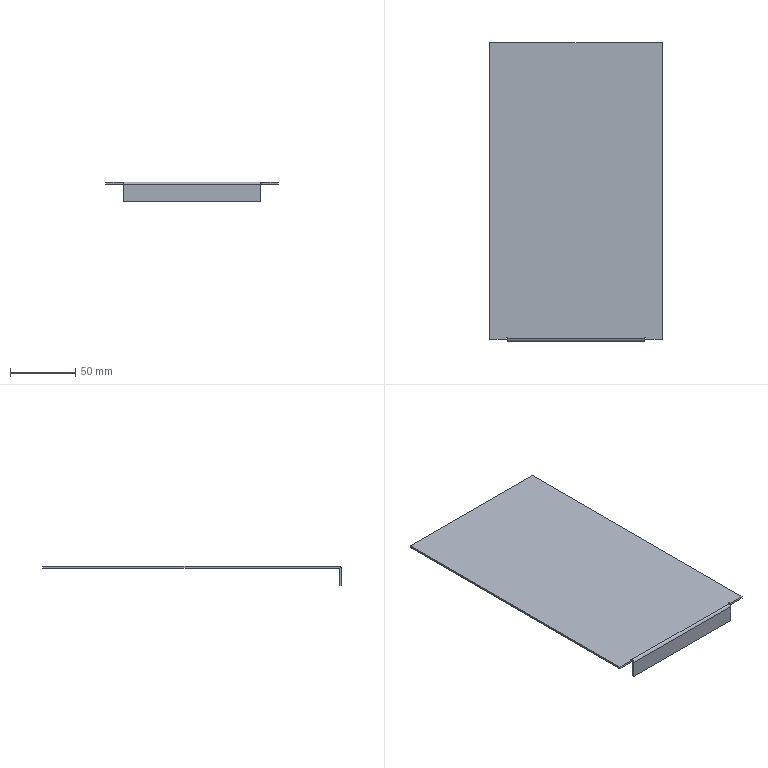Part | STEP file | X Motor Cover 1-1 | 1 solid | 18 faces | box 132 x 228.5 x 15 mm | volume 47221 mm3 | plane 14 | cylinder 4 | commonest cylinder face diameters 0.75 x2 1 x1 4 x1
STEP:
#1=CARTESIAN_POINT('',(-39.22,-140.718,-1.5));
#2=VERTEX_POINT('',#1);
#3=CARTESIAN_POINT('',(-26.47,-140.718,-1.5));
#4=VERTEX_POINT('',#3);
#5=CARTESIAN_POINT('',(0.,-140.718,-1.5));
#6=DIRECTION('',(1.,0.,0.));
#7=VECTOR('',#6,1000.);
#8=LINE('',#5,#7);
#9=EDGE_CURVE('',#2,#4,#8,.T.);
#10=ORIENTED_EDGE('',*,*,#9,.F.);
#11=CARTESIAN_POINT('',(-39.22,86.282,-1.5));
#12=VERTEX_POINT('',#11);
#13=CARTESIAN_POINT('',(-39.22,0.,-1.5));
#14=DIRECTION('',(0.,-1.,0.));
#15=VECTOR('',#14,1000.);
#16=LINE('',#13,#15);
#17=EDGE_CURVE('',#12,#2,#16,.T.);
#18=ORIENTED_EDGE('',*,*,#17,.F.);
#19=CARTESIAN_POINT('',(92.78,86.282,-1.5));
#20=VERTEX_POINT('',#19);
#21=CARTESIAN_POINT('',(0.,86.282,-1.5));
#22=DIRECTION('',(-1.,0.,0.));
#23=VECTOR('',#22,1000.);
#24=LINE('',#21,#23);
#25=EDGE_CURVE('',#20,#12,#24,.T.);
#26=ORIENTED_EDGE('',*,*,#25,.F.);
#27=CARTESIAN_POINT('',(92.78,-140.718,-1.5));
#28=VERTEX_POINT('',#27);
#29=CARTESIAN_POINT('',(92.78,0.,-1.5));
#30=DIRECTION('',(0.,1.,0.));
#31=VECTOR('',#30,1000.);
#32=LINE('',#29,#31);
#33=EDGE_CURVE('',#28,#20,#32,.T.);
#34=ORIENTED_EDGE('',*,*,#33,.F.);
#35=CARTESIAN_POINT('',(80.03,-140.718,-1.5));
#36=VERTEX_POINT('',#35);
#37=CARTESIAN_POINT('',(0.,-140.718,-1.5));
#38=DIRECTION('',(1.,0.,0.));
#39=VECTOR('',#38,1000.);
#40=LINE('',#37,#39);
#41=EDGE_CURVE('',#36,#28,#40,.T.);
#42=ORIENTED_EDGE('',*,*,#41,.F.);
#43=CARTESIAN_POINT('',(80.03,-139.468,-1.5));
#44=VERTEX_POINT('',#43);
#45=CARTESIAN_POINT('',(80.03,0.,-1.5));
#46=DIRECTION('',(0.,-1.,0.));
#47=VECTOR('',#46,1000.);
#48=LINE('',#45,#47);
#49=EDGE_CURVE('',#44,#36,#48,.T.);
#50=ORIENTED_EDGE('',*,*,#49,.F.);
#51=CARTESIAN_POINT('',(79.28,-139.468,-1.5));
#52=VERTEX_POINT('',#51);
#53=CARTESIAN_POINT('',(79.655,-139.468,-1.5));
#54=DIRECTION('',(0.,0.,-1.));
#55=DIRECTION('',(1.,0.,0.));
#56=AXIS2_PLACEMENT_3D('',#53,#54,#55);
#57=CIRCLE('',#56,0.375);
#58=EDGE_CURVE('',#52,#44,#57,.T.);
#59=ORIENTED_EDGE('',*,*,#58,.F.);
#60=CARTESIAN_POINT('',(79.28,-140.218,-1.5));
#61=VERTEX_POINT('',#60);
#62=CARTESIAN_POINT('',(79.28,-140.218,-1.5));
#63=DIRECTION('',(0.,1.,0.));
#64=VECTOR('',#63,1000.);
#65=LINE('',#62,#64);
#66=EDGE_CURVE('',#61,#52,#65,.T.);
#67=ORIENTED_EDGE('',*,*,#66,.F.);
#68=CARTESIAN_POINT('',(-25.72,-140.218,-1.5));
#69=VERTEX_POINT('',#68);
#70=CARTESIAN_POINT('',(0.,-140.218,-1.5));
#71=DIRECTION('',(1.,0.,0.));
#72=VECTOR('',#71,1000.);
#73=LINE('',#70,#72);
#74=EDGE_CURVE('',#69,#61,#73,.T.);
#75=ORIENTED_EDGE('',*,*,#74,.F.);
#76=CARTESIAN_POINT('',(-25.72,-139.468,-1.5));
#77=VERTEX_POINT('',#76);
#78=CARTESIAN_POINT('',(-25.72,0.,-1.5));
#79=DIRECTION('',(0.,-1.,0.));
#80=VECTOR('',#79,1000.);
#81=LINE('',#78,#80);
#82=EDGE_CURVE('',#77,#69,#81,.T.);
#83=ORIENTED_EDGE('',*,*,#82,.F.);
#84=CARTESIAN_POINT('',(-26.47,-139.468,-1.5));
#85=VERTEX_POINT('',#84);
#86=CARTESIAN_POINT('',(-26.095,-139.468,-1.5));
#87=DIRECTION('',(0.,0.,-1.));
#88=DIRECTION('',(1.,0.,0.));
#89=AXIS2_PLACEMENT_3D('',#86,#87,#88);
#90=CIRCLE('',#89,0.375);
#91=EDGE_CURVE('',#85,#77,#90,.T.);
#92=ORIENTED_EDGE('',*,*,#91,.F.);
#93=CARTESIAN_POINT('',(-26.47,0.,-1.5));
#94=DIRECTION('',(0.,1.,0.));
#95=VECTOR('',#94,1000.);
#96=LINE('',#93,#95);
#97=EDGE_CURVE('',#4,#85,#96,.T.);
#98=ORIENTED_EDGE('',*,*,#97,.F.);
#99=EDGE_LOOP('',(#10,#18,#26,#34,#42,#50,#59,#67,#75,#83,#92,#98));
#100=FACE_OUTER_BOUND('',#99,.T.);
#101=CARTESIAN_POINT('',(0.,0.,-1.5));
#102=DIRECTION('',(0.,0.,1.));
#103=DIRECTION('',(1.,0.,0.));
#104=AXIS2_PLACEMENT_3D('',#101,#102,#103);
#105=PLANE('',#104);
#106=ADVANCED_FACE('',(#100),#105,.F.);
#107=ORIENTED_EDGE('',*,*,#97,.T.);
#108=CARTESIAN_POINT('',(-26.47,-139.468,0.));
#109=VERTEX_POINT('',#108);
#110=CARTESIAN_POINT('',(-26.47,-139.468,-1.5));
#111=DIRECTION('',(0.,0.,1.));
#112=VECTOR('',#111,1000.);
#113=LINE('',#110,#112);
#114=EDGE_CURVE('',#85,#109,#113,.T.);
#115=ORIENTED_EDGE('',*,*,#114,.T.);
#116=CARTESIAN_POINT('',(-26.47,-140.718,0.));
#117=VERTEX_POINT('',#116);
#118=CARTESIAN_POINT('',(-26.47,0.,0.));
#119=DIRECTION('',(0.,1.,0.));
#120=VECTOR('',#119,1000.);
#121=LINE('',#118,#120);
#122=EDGE_CURVE('',#117,#109,#121,.T.);
#123=ORIENTED_EDGE('',*,*,#122,.F.);
#124=CARTESIAN_POINT('',(-26.47,-140.718,-1.5));
#125=DIRECTION('',(0.,0.,-1.));
#126=VECTOR('',#125,1000.);
#127=LINE('',#124,#126);
#128=EDGE_CURVE('',#117,#4,#127,.T.);
#129=ORIENTED_EDGE('',*,*,#128,.T.);
#130=EDGE_LOOP('',(#107,#115,#123,#129));
#131=FACE_OUTER_BOUND('',#130,.T.);
#132=CARTESIAN_POINT('',(-26.47,-140.718,-1.5));
#133=DIRECTION('',(1.,0.,0.));
#134=DIRECTION('',(0.,0.,-1.));
#135=AXIS2_PLACEMENT_3D('',#132,#133,#134);
#136=PLANE('',#135);
#137=ADVANCED_FACE('',(#131),#136,.T.);
#138=CARTESIAN_POINT('',(-39.22,-140.718,0.));
#139=VERTEX_POINT('',#138);
#140=CARTESIAN_POINT('',(-39.22,-140.718,0.));
#141=DIRECTION('',(-1.,0.,0.));
#142=VECTOR('',#141,1000.);
#143=LINE('',#140,#142);
#144=EDGE_CURVE('',#117,#139,#143,.T.);
#145=ORIENTED_EDGE('',*,*,#144,.T.);
#146=CARTESIAN_POINT('',(-39.22,-140.718,-1.5));
#147=DIRECTION('',(0.,0.,-1.));
#148=VECTOR('',#147,1000.);
#149=LINE('',#146,#148);
#150=EDGE_CURVE('',#139,#2,#149,.T.);
#151=ORIENTED_EDGE('',*,*,#150,.T.);
#152=ORIENTED_EDGE('',*,*,#9,.T.);
#153=ORIENTED_EDGE('',*,*,#128,.F.);
#154=EDGE_LOOP('',(#145,#151,#152,#153));
#155=FACE_OUTER_BOUND('',#154,.T.);
#156=CARTESIAN_POINT('',(-39.22,-140.718,-1.5));
#157=DIRECTION('',(0.,-1.,0.));
#158=DIRECTION('',(0.,0.,-1.));
#159=AXIS2_PLACEMENT_3D('',#156,#157,#158);
#160=PLANE('',#159);
#161=ADVANCED_FACE('',(#155),#160,.T.);
#162=ORIENTED_EDGE('',*,*,#17,.T.);
#163=ORIENTED_EDGE('',*,*,#150,.F.);
#164=CARTESIAN_POINT('',(-39.22,86.282,0.));
#165=VERTEX_POINT('',#164);
#166=CARTESIAN_POINT('',(-39.22,86.282,0.));
#167=DIRECTION('',(0.,1.,0.));
#168=VECTOR('',#167,1000.);
#169=LINE('',#166,#168);
#170=EDGE_CURVE('',#139,#165,#169,.T.);
#171=ORIENTED_EDGE('',*,*,#170,.T.);
#172=CARTESIAN_POINT('',(-39.22,86.282,-1.5));
#173=DIRECTION('',(0.,0.,-1.));
#174=VECTOR('',#173,1000.);
#175=LINE('',#172,#174);
#176=EDGE_CURVE('',#165,#12,#175,.T.);
#177=ORIENTED_EDGE('',*,*,#176,.T.);
#178=EDGE_LOOP('',(#162,#163,#171,#177));
#179=FACE_OUTER_BOUND('',#178,.T.);
#180=CARTESIAN_POINT('',(-39.22,86.282,-1.5));
#181=DIRECTION('',(-1.,0.,0.));
#182=DIRECTION('',(0.,-1.,0.));
#183=AXIS2_PLACEMENT_3D('',#180,#181,#182);
#184=PLANE('',#183);
#185=ADVANCED_FACE('',(#179),#184,.T.);
#186=ORIENTED_EDGE('',*,*,#25,.T.);
#187=ORIENTED_EDGE('',*,*,#176,.F.);
#188=CARTESIAN_POINT('',(92.78,86.282,0.));
#189=VERTEX_POINT('',#188);
#190=CARTESIAN_POINT('',(-39.22,86.282,0.));
#191=DIRECTION('',(1.,0.,0.));
#192=VECTOR('',#191,1000.);
#193=LINE('',#190,#192);
#194=EDGE_CURVE('',#165,#189,#193,.T.);
#195=ORIENTED_EDGE('',*,*,#194,.T.);
#196=CARTESIAN_POINT('',(92.78,86.282,-1.5));
#197=DIRECTION('',(0.,0.,-1.));
#198=VECTOR('',#197,1000.);
#199=LINE('',#196,#198);
#200=EDGE_CURVE('',#189,#20,#199,.T.);
#201=ORIENTED_EDGE('',*,*,#200,.T.);
#202=EDGE_LOOP('',(#186,#187,#195,#201));
#203=FACE_OUTER_BOUND('',#202,.T.);
#204=CARTESIAN_POINT('',(-39.22,86.282,-1.5));
#205=DIRECTION('',(0.,1.,0.));
#206=DIRECTION('',(0.,0.,1.));
#207=AXIS2_PLACEMENT_3D('',#204,#205,#206);
#208=PLANE('',#207);
#209=ADVANCED_FACE('',(#203),#208,.T.);
#210=ORIENTED_EDGE('',*,*,#33,.T.);
#211=ORIENTED_EDGE('',*,*,#200,.F.);
#212=CARTESIAN_POINT('',(92.78,-140.718,0.));
#213=VERTEX_POINT('',#212);
#214=CARTESIAN_POINT('',(92.78,86.282,0.));
#215=DIRECTION('',(0.,-1.,0.));
#216=VECTOR('',#215,1000.);
#217=LINE('',#214,#216);
#218=EDGE_CURVE('',#189,#213,#217,.T.);
#219=ORIENTED_EDGE('',*,*,#218,.T.);
#220=CARTESIAN_POINT('',(92.78,-140.718,-1.5));
#221=DIRECTION('',(0.,0.,-1.));
#222=VECTOR('',#221,1000.);
#223=LINE('',#220,#222);
#224=EDGE_CURVE('',#213,#28,#223,.T.);
#225=ORIENTED_EDGE('',*,*,#224,.T.);
#226=EDGE_LOOP('',(#210,#211,#219,#225));
#227=FACE_OUTER_BOUND('',#226,.T.);
#228=CARTESIAN_POINT('',(92.78,86.282,-1.5));
#229=DIRECTION('',(1.,0.,0.));
#230=DIRECTION('',(0.,1.,0.));
#231=AXIS2_PLACEMENT_3D('',#228,#229,#230);
#232=PLANE('',#231);
#233=ADVANCED_FACE('',(#227),#232,.T.);
#234=ORIENTED_EDGE('',*,*,#41,.T.);
#235=ORIENTED_EDGE('',*,*,#224,.F.);
#236=CARTESIAN_POINT('',(80.03,-140.718,0.));
#237=VERTEX_POINT('',#236);
#238=CARTESIAN_POINT('',(-39.22,-140.718,0.));
#239=DIRECTION('',(-1.,0.,0.));
#240=VECTOR('',#239,1000.);
#241=LINE('',#238,#240);
#242=EDGE_CURVE('',#213,#237,#241,.T.);
#243=ORIENTED_EDGE('',*,*,#242,.T.);
#244=CARTESIAN_POINT('',(80.03,-140.718,-1.5));
#245=DIRECTION('',(0.,0.,-1.));
#246=VECTOR('',#245,1000.);
#247=LINE('',#244,#246);
#248=EDGE_CURVE('',#237,#36,#247,.T.);
#249=ORIENTED_EDGE('',*,*,#248,.T.);
#250=EDGE_LOOP('',(#234,#235,#243,#249));
#251=FACE_OUTER_BOUND('',#250,.T.);
#252=CARTESIAN_POINT('',(-39.22,-140.718,-1.5));
#253=DIRECTION('',(0.,-1.,0.));
#254=DIRECTION('',(0.,0.,-1.));
#255=AXIS2_PLACEMENT_3D('',#252,#253,#254);
#256=PLANE('',#255);
#257=ADVANCED_FACE('',(#251),#256,.T.);
#258=ORIENTED_EDGE('',*,*,#49,.T.);
#259=ORIENTED_EDGE('',*,*,#248,.F.);
#260=CARTESIAN_POINT('',(80.03,-139.468,0.));
#261=VERTEX_POINT('',#260);
#262=CARTESIAN_POINT('',(80.03,-139.468,0.));
#263=DIRECTION('',(0.,1.,0.));
#264=VECTOR('',#263,1000.);
#265=LINE('',#262,#264);
#266=EDGE_CURVE('',#237,#261,#265,.T.);
#267=ORIENTED_EDGE('',*,*,#266,.T.);
#268=CARTESIAN_POINT('',(80.03,-139.468,-1.5));
#269=DIRECTION('',(0.,0.,-1.));
#270=VECTOR('',#269,1000.);
#271=LINE('',#268,#270);
#272=EDGE_CURVE('',#261,#44,#271,.T.);
#273=ORIENTED_EDGE('',*,*,#272,.T.);
#274=EDGE_LOOP('',(#258,#259,#267,#273));
#275=FACE_OUTER_BOUND('',#274,.T.);
#276=CARTESIAN_POINT('',(80.03,-139.468,-1.5));
#277=DIRECTION('',(-1.,0.,0.));
#278=DIRECTION('',(0.,0.,1.));
#279=AXIS2_PLACEMENT_3D('',#276,#277,#278);
#280=PLANE('',#279);
#281=ADVANCED_FACE('',(#275),#280,.T.);
#282=CARTESIAN_POINT('',(79.28,-139.468,0.));
#283=VERTEX_POINT('',#282);
#284=CARTESIAN_POINT('',(79.28,-139.468,-1.5));
#285=DIRECTION('',(0.,0.,1.));
#286=VECTOR('',#285,1000.);
#287=LINE('',#284,#286);
#288=EDGE_CURVE('',#52,#283,#287,.T.);
#289=ORIENTED_EDGE('',*,*,#288,.F.);
#290=ORIENTED_EDGE('',*,*,#58,.T.);
#291=ORIENTED_EDGE('',*,*,#272,.F.);
#292=CARTESIAN_POINT('',(79.655,-139.468,0.));
#293=DIRECTION('',(0.,0.,-1.));
#294=DIRECTION('',(1.,0.,0.));
#295=AXIS2_PLACEMENT_3D('',#292,#293,#294);
#296=CIRCLE('',#295,0.375);
#297=EDGE_CURVE('',#283,#261,#296,.T.);
#298=ORIENTED_EDGE('',*,*,#297,.F.);
#299=EDGE_LOOP('',(#289,#290,#291,#298));
#300=FACE_OUTER_BOUND('',#299,.T.);
#301=CARTESIAN_POINT('',(79.655,-139.468,-1.5));
#302=DIRECTION('',(0.,0.,1.));
#303=DIRECTION('',(1.,0.,0.));
#304=AXIS2_PLACEMENT_3D('',#301,#302,#303);
#305=CYLINDRICAL_SURFACE('',#304,0.375);
#306=ADVANCED_FACE('',(#300),#305,.F.);
#307=CARTESIAN_POINT('',(79.28,-140.718,-2.));
#308=VERTEX_POINT('',#307);
#309=CARTESIAN_POINT('',(79.28,-140.218,-2.));
#310=DIRECTION('',(-1.,0.,0.));
#311=DIRECTION('',(0.,0.,1.));
#312=AXIS2_PLACEMENT_3D('',#309,#310,#311);
#313=CIRCLE('',#312,0.5);
#314=EDGE_CURVE('',#308,#61,#313,.T.);
#315=ORIENTED_EDGE('',*,*,#314,.F.);
#316=CARTESIAN_POINT('',(-25.72,-140.718,-2.));
#317=VERTEX_POINT('',#316);
#318=CARTESIAN_POINT('',(-25.72,-140.718,-2.));
#319=DIRECTION('',(1.,0.,0.));
#320=VECTOR('',#319,1000.);
#321=LINE('',#318,#320);
#322=EDGE_CURVE('',#317,#308,#321,.T.);
#323=ORIENTED_EDGE('',*,*,#322,.F.);
#324=CARTESIAN_POINT('',(-25.72,-140.218,-2.));
#325=DIRECTION('',(-1.,0.,0.));
#326=DIRECTION('',(0.,0.,1.));
#327=AXIS2_PLACEMENT_3D('',#324,#325,#326);
#328=CIRCLE('',#327,0.5);
#329=EDGE_CURVE('',#317,#69,#328,.T.);
#330=ORIENTED_EDGE('',*,*,#329,.T.);
#331=ORIENTED_EDGE('',*,*,#74,.T.);
#332=EDGE_LOOP('',(#315,#323,#330,#331));
#333=FACE_OUTER_BOUND('',#332,.T.);
#334=CARTESIAN_POINT('',(-25.72,-140.218,-2.));
#335=DIRECTION('',(-1.,0.,0.));
#336=DIRECTION('',(0.,0.,1.));
#337=AXIS2_PLACEMENT_3D('',#334,#335,#336);
#338=CYLINDRICAL_SURFACE('',#337,0.5);
#339=ADVANCED_FACE('',(#333),#338,.F.);
#340=ORIENTED_EDGE('',*,*,#82,.T.);
#341=ORIENTED_EDGE('',*,*,#329,.F.);
#342=CARTESIAN_POINT('',(-25.72,-140.718,-15.));
#343=VERTEX_POINT('',#342);
#344=CARTESIAN_POINT('',(-25.72,-140.718,0.));
#345=DIRECTION('',(0.,0.,-1.));
#346=VECTOR('',#345,1000.);
#347=LINE('',#344,#346);
#348=EDGE_CURVE('',#317,#343,#347,.T.);
#349=ORIENTED_EDGE('',*,*,#348,.T.);
#350=CARTESIAN_POINT('',(-25.72,-142.218,-15.));
#351=VERTEX_POINT('',#350);
#352=CARTESIAN_POINT('',(-25.72,-142.218,-15.));
#353=DIRECTION('',(0.,1.,0.));
#354=VECTOR('',#353,1000.);
#355=LINE('',#352,#354);
#356=EDGE_CURVE('',#351,#343,#355,.T.);
#357=ORIENTED_EDGE('',*,*,#356,.F.);
#358=CARTESIAN_POINT('',(-25.72,-142.218,-2.));
#359=VERTEX_POINT('',#358);
#360=CARTESIAN_POINT('',(-25.72,-142.218,-1.5));
#361=DIRECTION('',(0.,0.,1.));
#362=VECTOR('',#361,1000.);
#363=LINE('',#360,#362);
#364=EDGE_CURVE('',#351,#359,#363,.T.);
#365=ORIENTED_EDGE('',*,*,#364,.T.);
#366=CARTESIAN_POINT('',(-25.72,-140.218,0.));
#367=VERTEX_POINT('',#366);
#368=CARTESIAN_POINT('',(-25.72,-140.218,-2.));
#369=DIRECTION('',(1.,0.,0.));
#370=DIRECTION('',(0.,0.,1.));
#371=AXIS2_PLACEMENT_3D('',#368,#369,#370);
#372=CIRCLE('',#371,2.);
#373=EDGE_CURVE('',#367,#359,#372,.T.);
#374=ORIENTED_EDGE('',*,*,#373,.F.);
#375=CARTESIAN_POINT('',(-25.72,-139.468,0.));
#376=VERTEX_POINT('',#375);
#377=CARTESIAN_POINT('',(-25.72,-139.468,0.));
#378=DIRECTION('',(0.,1.,0.));
#379=VECTOR('',#378,1000.);
#380=LINE('',#377,#379);
#381=EDGE_CURVE('',#367,#376,#380,.T.);
#382=ORIENTED_EDGE('',*,*,#381,.T.);
#383=CARTESIAN_POINT('',(-25.72,-139.468,-1.5));
#384=DIRECTION('',(0.,0.,-1.));
#385=VECTOR('',#384,1000.);
#386=LINE('',#383,#385);
#387=EDGE_CURVE('',#376,#77,#386,.T.);
#388=ORIENTED_EDGE('',*,*,#387,.T.);
#389=EDGE_LOOP('',(#340,#341,#349,#357,#365,#374,#382,#388));
#390=FACE_OUTER_BOUND('',#389,.T.);
#391=CARTESIAN_POINT('',(-25.72,-139.468,-1.5));
#392=DIRECTION('',(-1.,0.,0.));
#393=DIRECTION('',(0.,0.,1.));
#394=AXIS2_PLACEMENT_3D('',#391,#392,#393);
#395=PLANE('',#394);
#396=ADVANCED_FACE('',(#390),#395,.T.);
#397=ORIENTED_EDGE('',*,*,#114,.F.);
#398=ORIENTED_EDGE('',*,*,#91,.T.);
#399=ORIENTED_EDGE('',*,*,#387,.F.);
#400=CARTESIAN_POINT('',(-26.095,-139.468,0.));
#401=DIRECTION('',(0.,0.,-1.));
#402=DIRECTION('',(1.,0.,0.));
#403=AXIS2_PLACEMENT_3D('',#400,#401,#402);
#404=CIRCLE('',#403,0.375);
#405=EDGE_CURVE('',#109,#376,#404,.T.);
#406=ORIENTED_EDGE('',*,*,#405,.F.);
#407=EDGE_LOOP('',(#397,#398,#399,#406));
#408=FACE_OUTER_BOUND('',#407,.T.);
#409=CARTESIAN_POINT('',(-26.095,-139.468,-1.5));
#410=DIRECTION('',(0.,0.,1.));
#411=DIRECTION('',(1.,0.,0.));
#412=AXIS2_PLACEMENT_3D('',#409,#410,#411);
#413=CYLINDRICAL_SURFACE('',#412,0.375);
#414=ADVANCED_FACE('',(#408),#413,.F.);
#415=ORIENTED_EDGE('',*,*,#194,.F.);
#416=ORIENTED_EDGE('',*,*,#170,.F.);
#417=ORIENTED_EDGE('',*,*,#144,.F.);
#418=ORIENTED_EDGE('',*,*,#122,.T.);
#419=ORIENTED_EDGE('',*,*,#405,.T.);
#420=ORIENTED_EDGE('',*,*,#381,.F.);
#421=CARTESIAN_POINT('',(79.28,-140.218,0.));
#422=VERTEX_POINT('',#421);
#423=CARTESIAN_POINT('',(0.,-140.218,0.));
#424=DIRECTION('',(1.,0.,0.));
#425=VECTOR('',#424,1000.);
#426=LINE('',#423,#425);
#427=EDGE_CURVE('',#367,#422,#426,.T.);
#428=ORIENTED_EDGE('',*,*,#427,.T.);
#429=CARTESIAN_POINT('',(79.28,0.,0.));
#430=DIRECTION('',(0.,1.,0.));
#431=VECTOR('',#430,1000.);
#432=LINE('',#429,#431);
#433=EDGE_CURVE('',#422,#283,#432,.T.);
#434=ORIENTED_EDGE('',*,*,#433,.T.);
#435=ORIENTED_EDGE('',*,*,#297,.T.);
#436=ORIENTED_EDGE('',*,*,#266,.F.);
#437=ORIENTED_EDGE('',*,*,#242,.F.);
#438=ORIENTED_EDGE('',*,*,#218,.F.);
#439=EDGE_LOOP('',(#415,#416,#417,#418,#419,#420,#428,#434,#435,#436,#437,#438));
#440=FACE_OUTER_BOUND('',#439,.T.);
#441=CARTESIAN_POINT('',(0.,0.,0.));
#442=DIRECTION('',(0.,0.,1.));
#443=DIRECTION('',(1.,0.,0.));
#444=AXIS2_PLACEMENT_3D('',#441,#442,#443);
#445=PLANE('',#444);
#446=ADVANCED_FACE('',(#440),#445,.T.);
#447=ORIENTED_EDGE('',*,*,#66,.T.);
#448=ORIENTED_EDGE('',*,*,#288,.T.);
#449=ORIENTED_EDGE('',*,*,#433,.F.);
#450=CARTESIAN_POINT('',(79.28,-142.218,-2.));
#451=VERTEX_POINT('',#450);
#452=CARTESIAN_POINT('',(79.28,-140.218,-2.));
#453=DIRECTION('',(-1.,0.,0.));
#454=DIRECTION('',(0.,0.,1.));
#455=AXIS2_PLACEMENT_3D('',#452,#453,#454);
#456=CIRCLE('',#455,2.);
#457=EDGE_CURVE('',#451,#422,#456,.T.);
#458=ORIENTED_EDGE('',*,*,#457,.F.);
#459=CARTESIAN_POINT('',(79.28,-142.218,-15.));
#460=VERTEX_POINT('',#459);
#461=CARTESIAN_POINT('',(79.28,-142.218,-15.));
#462=DIRECTION('',(0.,0.,-1.));
#463=VECTOR('',#462,1000.);
#464=LINE('',#461,#463);
#465=EDGE_CURVE('',#451,#460,#464,.T.);
#466=ORIENTED_EDGE('',*,*,#465,.T.);
#467=CARTESIAN_POINT('',(79.28,-140.718,-15.));
#468=VERTEX_POINT('',#467);
#469=CARTESIAN_POINT('',(79.28,-142.218,-15.));
#470=DIRECTION('',(0.,1.,0.));
#471=VECTOR('',#470,1000.);
#472=LINE('',#469,#471);
#473=EDGE_CURVE('',#460,#468,#472,.T.);
#474=ORIENTED_EDGE('',*,*,#473,.T.);
#475=CARTESIAN_POINT('',(79.28,-140.718,0.));
#476=DIRECTION('',(0.,0.,1.));
#477=VECTOR('',#476,1000.);
#478=LINE('',#475,#477);
#479=EDGE_CURVE('',#468,#308,#478,.T.);
#480=ORIENTED_EDGE('',*,*,#479,.T.);
#481=ORIENTED_EDGE('',*,*,#314,.T.);
#482=EDGE_LOOP('',(#447,#448,#449,#458,#466,#474,#480,#481));
#483=FACE_OUTER_BOUND('',#482,.T.);
#484=CARTESIAN_POINT('',(79.28,-140.218,-1.5));
#485=DIRECTION('',(1.,0.,0.));
#486=DIRECTION('',(0.,0.,-1.));
#487=AXIS2_PLACEMENT_3D('',#484,#485,#486);
#488=PLANE('',#487);
#489=ADVANCED_FACE('',(#483),#488,.T.);
#490=ORIENTED_EDGE('',*,*,#479,.F.);
#491=CARTESIAN_POINT('',(0.,-140.718,-15.));
#492=DIRECTION('',(1.,0.,0.));
#493=VECTOR('',#492,1000.);
#494=LINE('',#491,#493);
#495=EDGE_CURVE('',#343,#468,#494,.T.);
#496=ORIENTED_EDGE('',*,*,#495,.F.);
#497=ORIENTED_EDGE('',*,*,#348,.F.);
#498=ORIENTED_EDGE('',*,*,#322,.T.);
#499=EDGE_LOOP('',(#490,#496,#497,#498));
#500=FACE_OUTER_BOUND('',#499,.T.);
#501=CARTESIAN_POINT('',(0.,-140.718,0.));
#502=DIRECTION('',(0.,-1.,0.));
#503=DIRECTION('',(0.,0.,-1.));
#504=AXIS2_PLACEMENT_3D('',#501,#502,#503);
#505=PLANE('',#504);
#506=ADVANCED_FACE('',(#500),#505,.F.);
#507=CARTESIAN_POINT('',(-25.72,-142.218,-2.));
#508=DIRECTION('',(1.,0.,0.));
#509=VECTOR('',#508,1000.);
#510=LINE('',#507,#509);
#511=EDGE_CURVE('',#359,#451,#510,.T.);
#512=ORIENTED_EDGE('',*,*,#511,.T.);
#513=ORIENTED_EDGE('',*,*,#457,.T.);
#514=ORIENTED_EDGE('',*,*,#427,.F.);
#515=ORIENTED_EDGE('',*,*,#373,.T.);
#516=EDGE_LOOP('',(#512,#513,#514,#515));
#517=FACE_OUTER_BOUND('',#516,.T.);
#518=CARTESIAN_POINT('',(-25.72,-140.218,-2.));
#519=DIRECTION('',(-1.,0.,0.));
#520=DIRECTION('',(0.,0.,1.));
#521=AXIS2_PLACEMENT_3D('',#518,#519,#520);
#522=CYLINDRICAL_SURFACE('',#521,2.);
#523=ADVANCED_FACE('',(#517),#522,.T.);
#524=CARTESIAN_POINT('',(-25.72,-142.218,-15.));
#525=DIRECTION('',(-1.,0.,0.));
#526=VECTOR('',#525,1000.);
#527=LINE('',#524,#526);
#528=EDGE_CURVE('',#460,#351,#527,.T.);
#529=ORIENTED_EDGE('',*,*,#528,.T.);
#530=ORIENTED_EDGE('',*,*,#356,.T.);
#531=ORIENTED_EDGE('',*,*,#495,.T.);
#532=ORIENTED_EDGE('',*,*,#473,.F.);
#533=EDGE_LOOP('',(#529,#530,#531,#532));
#534=FACE_OUTER_BOUND('',#533,.T.);
#535=CARTESIAN_POINT('',(-25.72,-142.218,-15.));
#536=DIRECTION('',(0.,0.,-1.));
#537=DIRECTION('',(0.,1.,0.));
#538=AXIS2_PLACEMENT_3D('',#535,#536,#537);
#539=PLANE('',#538);
#540=ADVANCED_FACE('',(#534),#539,.T.);
#541=ORIENTED_EDGE('',*,*,#364,.F.);
#542=ORIENTED_EDGE('',*,*,#528,.F.);
#543=ORIENTED_EDGE('',*,*,#465,.F.);
#544=ORIENTED_EDGE('',*,*,#511,.F.);
#545=EDGE_LOOP('',(#541,#542,#543,#544));
#546=FACE_OUTER_BOUND('',#545,.T.);
#547=CARTESIAN_POINT('',(0.,-142.218,0.));
#548=DIRECTION('',(0.,-1.,0.));
#549=DIRECTION('',(0.,0.,-1.));
#550=AXIS2_PLACEMENT_3D('',#547,#548,#549);
#551=PLANE('',#550);
#552=ADVANCED_FACE('',(#546),#551,.T.);
#553=CLOSED_SHELL('',(#106,#137,#161,#185,#209,#233,#257,#281,#306,#339,#396,#414,#446,#489,#506,#523,#540,#552));
#554=MANIFOLD_SOLID_BREP('',#553);
#555=CARTESIAN_POINT('',(0.,0.,0.));
#556=DIRECTION('',(0.,0.,1.));
#557=DIRECTION('',(1.,0.,0.));
#558=AXIS2_PLACEMENT_3D('',#555,#556,#557);
#559=(LENGTH_UNIT()NAMED_UNIT(*)SI_UNIT(.MILLI.,.METRE.));
#560=UNCERTAINTY_MEASURE_WITH_UNIT(LENGTH_MEASURE(0.00001),#559,'','');
#561=(NAMED_UNIT(*)PLANE_ANGLE_UNIT()SI_UNIT($,.RADIAN.));
#562=(NAMED_UNIT(*)SI_UNIT($,.STERADIAN.)SOLID_ANGLE_UNIT());
#563=(GEOMETRIC_REPRESENTATION_CONTEXT(3)GLOBAL_UNCERTAINTY_ASSIGNED_CONTEXT((#560))GLOBAL_UNIT_ASSIGNED_CONTEXT((#559,#561,#562))REPRESENTATION_CONTEXT('',''));
#564=ADVANCED_BREP_SHAPE_REPRESENTATION('',(#554,#558),#563);